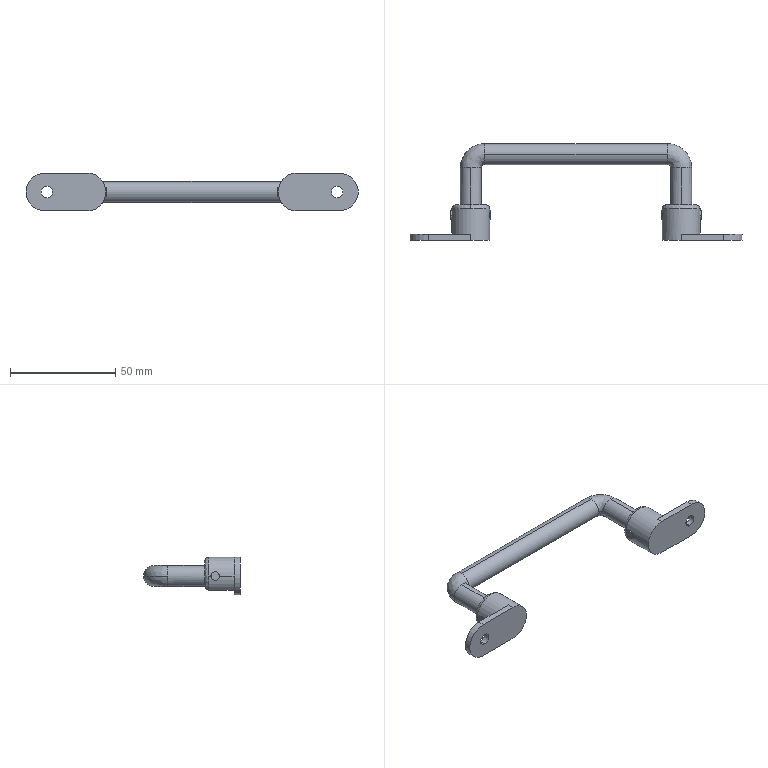Part | SolidWorks | features BaseBody 5 | 5 solids | 69 faces | box 158 x 46 x 18 mm | volume 18569 mm3 | cylinder 38 | plane 18 | spline 13 | commonest cylinder face diameters 4 x16 18 x8 10 x6 5.5 x4 14 x4